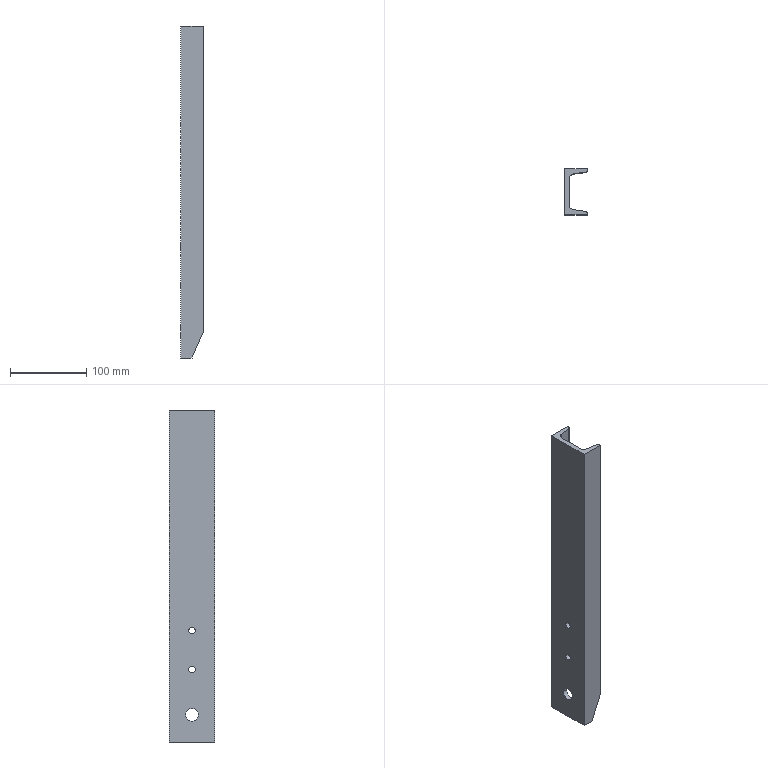Part | SolidWorks | features ICE 3, Extrusion 1 | 1 solid | 22 faces | box 30 x 60 x 435 mm | volume 272325 mm3 | plane 12 | cylinder 10 | commonest cylinder face diameters 8.5 x4 6 x2 12 x2 17 x2
STEP:
#1=CARTESIAN_POINT('',(-24.,-25.75,95.));
#2=VERTEX_POINT('',#1);
#3=CARTESIAN_POINT('',(-24.,-34.25,95.));
#4=VERTEX_POINT('',#3);
#5=CARTESIAN_POINT('',(-24.,-30.,95.));
#6=DIRECTION('',(-1.,0.,0.));
#7=DIRECTION('',(0.,0.,1.));
#8=AXIS2_PLACEMENT_3D('',#5,#6,#7);
#9=CIRCLE('',#8,4.25);
#10=EDGE_CURVE('',#2,#4,#9,.T.);
#11=ORIENTED_EDGE('',*,*,#10,.F.);
#12=CARTESIAN_POINT('',(-30.,-25.75,95.));
#13=VERTEX_POINT('',#12);
#14=CARTESIAN_POINT('',(405.,-25.75,95.));
#15=DIRECTION('',(-1.,0.,0.));
#16=VECTOR('',#15,1000.);
#17=LINE('',#14,#16);
#18=EDGE_CURVE('',#2,#13,#17,.T.);
#19=ORIENTED_EDGE('',*,*,#18,.T.);
#20=CARTESIAN_POINT('',(-30.,-34.25,95.));
#21=VERTEX_POINT('',#20);
#22=CARTESIAN_POINT('',(-30.,-30.,95.));
#23=DIRECTION('',(-1.,0.,0.));
#24=DIRECTION('',(0.,-1.,0.));
#25=AXIS2_PLACEMENT_3D('',#22,#23,#24);
#26=CIRCLE('',#25,4.25);
#27=EDGE_CURVE('',#13,#21,#26,.T.);
#28=ORIENTED_EDGE('',*,*,#27,.T.);
#29=CARTESIAN_POINT('',(405.,-34.25,95.));
#30=DIRECTION('',(-1.,0.,0.));
#31=VECTOR('',#30,1000.);
#32=LINE('',#29,#31);
#33=EDGE_CURVE('',#4,#21,#32,.T.);
#34=ORIENTED_EDGE('',*,*,#33,.F.);
#35=EDGE_LOOP('',(#11,#19,#28,#34));
#36=FACE_OUTER_BOUND('',#35,.T.);
#37=CARTESIAN_POINT('',(405.,-30.,95.));
#38=DIRECTION('',(-1.,0.,0.));
#39=DIRECTION('',(0.,-1.,0.));
#40=AXIS2_PLACEMENT_3D('',#37,#38,#39);
#41=CYLINDRICAL_SURFACE('',#40,4.25);
#42=ADVANCED_FACE('',(#36),#41,.F.);
#43=CARTESIAN_POINT('',(-24.,-25.75,146.));
#44=VERTEX_POINT('',#43);
#45=CARTESIAN_POINT('',(-24.,-34.25,146.));
#46=VERTEX_POINT('',#45);
#47=CARTESIAN_POINT('',(-24.,-30.,146.));
#48=DIRECTION('',(-1.,0.,0.));
#49=DIRECTION('',(0.,0.,1.));
#50=AXIS2_PLACEMENT_3D('',#47,#48,#49);
#51=CIRCLE('',#50,4.25);
#52=EDGE_CURVE('',#44,#46,#51,.T.);
#53=ORIENTED_EDGE('',*,*,#52,.F.);
#54=CARTESIAN_POINT('',(-30.,-25.75,146.));
#55=VERTEX_POINT('',#54);
#56=CARTESIAN_POINT('',(405.,-25.75,146.));
#57=DIRECTION('',(-1.,0.,0.));
#58=VECTOR('',#57,1000.);
#59=LINE('',#56,#58);
#60=EDGE_CURVE('',#44,#55,#59,.T.);
#61=ORIENTED_EDGE('',*,*,#60,.T.);
#62=CARTESIAN_POINT('',(-30.,-34.25,146.));
#63=VERTEX_POINT('',#62);
#64=CARTESIAN_POINT('',(-30.,-30.,146.));
#65=DIRECTION('',(-1.,0.,0.));
#66=DIRECTION('',(0.,-1.,0.));
#67=AXIS2_PLACEMENT_3D('',#64,#65,#66);
#68=CIRCLE('',#67,4.25);
#69=EDGE_CURVE('',#55,#63,#68,.T.);
#70=ORIENTED_EDGE('',*,*,#69,.T.);
#71=CARTESIAN_POINT('',(405.,-34.25,146.));
#72=DIRECTION('',(-1.,0.,0.));
#73=VECTOR('',#72,1000.);
#74=LINE('',#71,#73);
#75=EDGE_CURVE('',#46,#63,#74,.T.);
#76=ORIENTED_EDGE('',*,*,#75,.F.);
#77=EDGE_LOOP('',(#53,#61,#70,#76));
#78=FACE_OUTER_BOUND('',#77,.T.);
#79=CARTESIAN_POINT('',(405.,-30.,146.));
#80=DIRECTION('',(-1.,0.,0.));
#81=DIRECTION('',(0.,-1.,0.));
#82=AXIS2_PLACEMENT_3D('',#79,#80,#81);
#83=CYLINDRICAL_SURFACE('',#82,4.25);
#84=ADVANCED_FACE('',(#78),#83,.F.);
#85=CARTESIAN_POINT('',(-24.,-21.5,35.5));
#86=VERTEX_POINT('',#85);
#87=CARTESIAN_POINT('',(-24.,-38.5,35.5));
#88=VERTEX_POINT('',#87);
#89=CARTESIAN_POINT('',(-24.,-30.,35.5));
#90=DIRECTION('',(-1.,0.,0.));
#91=DIRECTION('',(0.,0.,1.));
#92=AXIS2_PLACEMENT_3D('',#89,#90,#91);
#93=CIRCLE('',#92,8.5);
#94=EDGE_CURVE('',#86,#88,#93,.T.);
#95=ORIENTED_EDGE('',*,*,#94,.F.);
#96=CARTESIAN_POINT('',(-30.,-21.5,35.5));
#97=VERTEX_POINT('',#96);
#98=CARTESIAN_POINT('',(405.,-21.5,35.5));
#99=DIRECTION('',(-1.,0.,0.));
#100=VECTOR('',#99,1000.);
#101=LINE('',#98,#100);
#102=EDGE_CURVE('',#86,#97,#101,.T.);
#103=ORIENTED_EDGE('',*,*,#102,.T.);
#104=CARTESIAN_POINT('',(-30.,-38.5,35.5));
#105=VERTEX_POINT('',#104);
#106=CARTESIAN_POINT('',(-30.,-30.,35.5));
#107=DIRECTION('',(-1.,0.,0.));
#108=DIRECTION('',(0.,-1.,0.));
#109=AXIS2_PLACEMENT_3D('',#106,#107,#108);
#110=CIRCLE('',#109,8.5);
#111=EDGE_CURVE('',#97,#105,#110,.T.);
#112=ORIENTED_EDGE('',*,*,#111,.T.);
#113=CARTESIAN_POINT('',(405.,-38.5,35.5));
#114=DIRECTION('',(-1.,0.,0.));
#115=VECTOR('',#114,1000.);
#116=LINE('',#113,#115);
#117=EDGE_CURVE('',#88,#105,#116,.T.);
#118=ORIENTED_EDGE('',*,*,#117,.F.);
#119=EDGE_LOOP('',(#95,#103,#112,#118));
#120=FACE_OUTER_BOUND('',#119,.T.);
#121=CARTESIAN_POINT('',(405.,-30.,35.5));
#122=DIRECTION('',(-1.,0.,0.));
#123=DIRECTION('',(0.,-1.,0.));
#124=AXIS2_PLACEMENT_3D('',#121,#122,#123);
#125=CYLINDRICAL_SURFACE('',#124,8.5);
#126=ADVANCED_FACE('',(#120),#125,.F.);
#127=CARTESIAN_POINT('',(0.,-1.284,435.));
#128=VERTEX_POINT('',#127);
#129=CARTESIAN_POINT('',(0.,-1.284,35.));
#130=VERTEX_POINT('',#129);
#131=CARTESIAN_POINT('',(0.,-1.284,435.));
#132=DIRECTION('',(0.,0.,-1.));
#133=VECTOR('',#132,1000.);
#134=LINE('',#131,#133);
#135=EDGE_CURVE('',#128,#130,#134,.T.);
#136=ORIENTED_EDGE('',*,*,#135,.T.);
#137=CARTESIAN_POINT('',(0.,0.,35.));
#138=VERTEX_POINT('',#137);
#139=CARTESIAN_POINT('',(0.,-435.,35.));
#140=DIRECTION('',(0.,1.,0.));
#141=VECTOR('',#140,1000.);
#142=LINE('',#139,#141);
#143=EDGE_CURVE('',#130,#138,#142,.T.);
#144=ORIENTED_EDGE('',*,*,#143,.T.);
#145=CARTESIAN_POINT('',(0.,0.,435.));
#146=VERTEX_POINT('',#145);
#147=CARTESIAN_POINT('',(0.,0.,435.));
#148=DIRECTION('',(0.,0.,-1.));
#149=VECTOR('',#148,1000.);
#150=LINE('',#147,#149);
#151=EDGE_CURVE('',#146,#138,#150,.T.);
#152=ORIENTED_EDGE('',*,*,#151,.F.);
#153=CARTESIAN_POINT('',(0.,-1.284,435.));
#154=DIRECTION('',(0.,1.,0.));
#155=VECTOR('',#154,1000.);
#156=LINE('',#153,#155);
#157=EDGE_CURVE('',#128,#146,#156,.T.);
#158=ORIENTED_EDGE('',*,*,#157,.F.);
#159=EDGE_LOOP('',(#136,#144,#152,#158));
#160=FACE_OUTER_BOUND('',#159,.T.);
#161=CARTESIAN_POINT('',(0.,-1.284,435.));
#162=DIRECTION('',(-1.,0.,0.));
#163=DIRECTION('',(0.,0.,1.));
#164=AXIS2_PLACEMENT_3D('',#161,#162,#163);
#165=PLANE('',#164);
#166=ADVANCED_FACE('',(#160),#165,.F.);
#167=ORIENTED_EDGE('',*,*,#151,.T.);
#168=CARTESIAN_POINT('',(-15.,0.,0.));
#169=VERTEX_POINT('',#168);
#170=CARTESIAN_POINT('',(0.,0.,35.));
#171=DIRECTION('',(0.3939,0.,0.9191));
#172=VECTOR('',#171,1000.);
#173=LINE('',#170,#172);
#174=EDGE_CURVE('',#169,#138,#173,.T.);
#175=ORIENTED_EDGE('',*,*,#174,.F.);
#176=CARTESIAN_POINT('',(-30.,0.,0.));
#177=VERTEX_POINT('',#176);
#178=CARTESIAN_POINT('',(0.,0.,0.));
#179=DIRECTION('',(-1.,0.,0.));
#180=VECTOR('',#179,1000.);
#181=LINE('',#178,#180);
#182=EDGE_CURVE('',#169,#177,#181,.T.);
#183=ORIENTED_EDGE('',*,*,#182,.T.);
#184=CARTESIAN_POINT('',(-30.,0.,435.));
#185=VERTEX_POINT('',#184);
#186=CARTESIAN_POINT('',(-30.,0.,435.));
#187=DIRECTION('',(0.,0.,-1.));
#188=VECTOR('',#187,1000.);
#189=LINE('',#186,#188);
#190=EDGE_CURVE('',#185,#177,#189,.T.);
#191=ORIENTED_EDGE('',*,*,#190,.F.);
#192=CARTESIAN_POINT('',(0.,0.,435.));
#193=DIRECTION('',(-1.,0.,0.));
#194=VECTOR('',#193,1000.);
#195=LINE('',#192,#194);
#196=EDGE_CURVE('',#146,#185,#195,.T.);
#197=ORIENTED_EDGE('',*,*,#196,.F.);
#198=EDGE_LOOP('',(#167,#175,#183,#191,#197));
#199=FACE_OUTER_BOUND('',#198,.T.);
#200=CARTESIAN_POINT('',(0.,0.,435.));
#201=DIRECTION('',(0.,-1.,0.));
#202=DIRECTION('',(1.,0.,0.));
#203=AXIS2_PLACEMENT_3D('',#200,#201,#202);
#204=PLANE('',#203);
#205=ADVANCED_FACE('',(#199),#204,.F.);
#206=CARTESIAN_POINT('',(-30.,-30.,95.));
#207=DIRECTION('',(-1.,0.,0.));
#208=DIRECTION('',(0.,-1.,0.));
#209=AXIS2_PLACEMENT_3D('',#206,#207,#208);
#210=CIRCLE('',#209,4.25);
#211=EDGE_CURVE('',#21,#13,#210,.T.);
#212=ORIENTED_EDGE('',*,*,#211,.F.);
#213=ORIENTED_EDGE('',*,*,#27,.F.);
#214=EDGE_LOOP('',(#212,#213));
#215=FACE_BOUND('',#214,.T.);
#216=CARTESIAN_POINT('',(-30.,-30.,146.));
#217=DIRECTION('',(-1.,0.,0.));
#218=DIRECTION('',(0.,-1.,0.));
#219=AXIS2_PLACEMENT_3D('',#216,#217,#218);
#220=CIRCLE('',#219,4.25);
#221=EDGE_CURVE('',#63,#55,#220,.T.);
#222=ORIENTED_EDGE('',*,*,#221,.F.);
#223=ORIENTED_EDGE('',*,*,#69,.F.);
#224=EDGE_LOOP('',(#222,#223));
#225=FACE_BOUND('',#224,.T.);
#226=CARTESIAN_POINT('',(-30.,-30.,35.5));
#227=DIRECTION('',(-1.,0.,0.));
#228=DIRECTION('',(0.,-1.,0.));
#229=AXIS2_PLACEMENT_3D('',#226,#227,#228);
#230=CIRCLE('',#229,8.5);
#231=EDGE_CURVE('',#105,#97,#230,.T.);
#232=ORIENTED_EDGE('',*,*,#231,.F.);
#233=ORIENTED_EDGE('',*,*,#111,.F.);
#234=EDGE_LOOP('',(#232,#233));
#235=FACE_BOUND('',#234,.T.);
#236=CARTESIAN_POINT('',(-30.,-60.,0.));
#237=VERTEX_POINT('',#236);
#238=CARTESIAN_POINT('',(-30.,0.,0.));
#239=DIRECTION('',(0.,-1.,0.));
#240=VECTOR('',#239,1000.);
#241=LINE('',#238,#240);
#242=EDGE_CURVE('',#177,#237,#241,.T.);
#243=ORIENTED_EDGE('',*,*,#242,.T.);
#244=CARTESIAN_POINT('',(-30.,-60.,435.));
#245=VERTEX_POINT('',#244);
#246=CARTESIAN_POINT('',(-30.,-60.,435.));
#247=DIRECTION('',(0.,0.,-1.));
#248=VECTOR('',#247,1000.);
#249=LINE('',#246,#248);
#250=EDGE_CURVE('',#245,#237,#249,.T.);
#251=ORIENTED_EDGE('',*,*,#250,.F.);
#252=CARTESIAN_POINT('',(-30.,0.,435.));
#253=DIRECTION('',(0.,-1.,0.));
#254=VECTOR('',#253,1000.);
#255=LINE('',#252,#254);
#256=EDGE_CURVE('',#185,#245,#255,.T.);
#257=ORIENTED_EDGE('',*,*,#256,.F.);
#258=ORIENTED_EDGE('',*,*,#190,.T.);
#259=EDGE_LOOP('',(#243,#251,#257,#258));
#260=FACE_OUTER_BOUND('',#259,.T.);
#261=CARTESIAN_POINT('',(-30.,0.,435.));
#262=DIRECTION('',(1.,0.,0.));
#263=DIRECTION('',(0.,1.,0.));
#264=AXIS2_PLACEMENT_3D('',#261,#262,#263);
#265=PLANE('',#264);
#266=ADVANCED_FACE('',(#215,#225,#235,#260),#265,.F.);
#267=CARTESIAN_POINT('',(-15.,-60.,0.));
#268=VERTEX_POINT('',#267);
#269=CARTESIAN_POINT('',(-30.,-60.,0.));
#270=DIRECTION('',(1.,0.,0.));
#271=VECTOR('',#270,1000.);
#272=LINE('',#269,#271);
#273=EDGE_CURVE('',#237,#268,#272,.T.);
#274=ORIENTED_EDGE('',*,*,#273,.T.);
#275=CARTESIAN_POINT('',(0.,-60.,35.));
#276=VERTEX_POINT('',#275);
#277=CARTESIAN_POINT('',(140.172,-60.,362.069));
#278=DIRECTION('',(0.3939,0.,0.9191));
#279=VECTOR('',#278,1000.);
#280=LINE('',#277,#279);
#281=EDGE_CURVE('',#268,#276,#280,.T.);
#282=ORIENTED_EDGE('',*,*,#281,.T.);
#283=CARTESIAN_POINT('',(0.,-60.,435.));
#284=VERTEX_POINT('',#283);
#285=CARTESIAN_POINT('',(0.,-60.,435.));
#286=DIRECTION('',(0.,0.,-1.));
#287=VECTOR('',#286,1000.);
#288=LINE('',#285,#287);
#289=EDGE_CURVE('',#284,#276,#288,.T.);
#290=ORIENTED_EDGE('',*,*,#289,.F.);
#291=CARTESIAN_POINT('',(-30.,-60.,435.));
#292=DIRECTION('',(1.,0.,0.));
#293=VECTOR('',#292,1000.);
#294=LINE('',#291,#293);
#295=EDGE_CURVE('',#245,#284,#294,.T.);
#296=ORIENTED_EDGE('',*,*,#295,.F.);
#297=ORIENTED_EDGE('',*,*,#250,.T.);
#298=EDGE_LOOP('',(#274,#282,#290,#296,#297));
#299=FACE_OUTER_BOUND('',#298,.T.);
#300=CARTESIAN_POINT('',(-30.,-60.,435.));
#301=DIRECTION('',(0.,1.,0.));
#302=DIRECTION('',(-1.,0.,0.));
#303=AXIS2_PLACEMENT_3D('',#300,#301,#302);
#304=PLANE('',#303);
#305=ADVANCED_FACE('',(#299),#304,.F.);
#306=ORIENTED_EDGE('',*,*,#289,.T.);
#307=CARTESIAN_POINT('',(0.,-58.716,35.));
#308=VERTEX_POINT('',#307);
#309=CARTESIAN_POINT('',(0.,-435.,35.));
#310=DIRECTION('',(0.,1.,0.));
#311=VECTOR('',#310,1000.);
#312=LINE('',#309,#311);
#313=EDGE_CURVE('',#276,#308,#312,.T.);
#314=ORIENTED_EDGE('',*,*,#313,.T.);
#315=CARTESIAN_POINT('',(0.,-58.716,435.));
#316=VERTEX_POINT('',#315);
#317=CARTESIAN_POINT('',(0.,-58.716,435.));
#318=DIRECTION('',(0.,0.,-1.));
#319=VECTOR('',#318,1000.);
#320=LINE('',#317,#319);
#321=EDGE_CURVE('',#316,#308,#320,.T.);
#322=ORIENTED_EDGE('',*,*,#321,.F.);
#323=CARTESIAN_POINT('',(0.,-60.,435.));
#324=DIRECTION('',(0.,1.,0.));
#325=VECTOR('',#324,1000.);
#326=LINE('',#323,#325);
#327=EDGE_CURVE('',#284,#316,#326,.T.);
#328=ORIENTED_EDGE('',*,*,#327,.F.);
#329=EDGE_LOOP('',(#306,#314,#322,#328));
#330=FACE_OUTER_BOUND('',#329,.T.);
#331=CARTESIAN_POINT('',(0.,-60.,435.));
#332=DIRECTION('',(-1.,0.,0.));
#333=DIRECTION('',(0.,0.,1.));
#334=AXIS2_PLACEMENT_3D('',#331,#332,#333);
#335=PLANE('',#334);
#336=ADVANCED_FACE('',(#330),#335,.F.);
#337=ORIENTED_EDGE('',*,*,#321,.T.);
#338=CARTESIAN_POINT('',(-2.582,-55.745,28.974));
#339=VERTEX_POINT('',#338);
#340=CARTESIAN_POINT('',(0.,-58.716,35.));
#341=CARTESIAN_POINT('',(0.,-57.147,35.));
#342=CARTESIAN_POINT('',(-1.029,-55.963,32.599));
#343=CARTESIAN_POINT('',(-2.582,-55.745,28.974));
#344=(BOUNDED_CURVE()B_SPLINE_CURVE(3,(#340,#341,#342,#343),.UNSPECIFIED.,.F.,.T.)B_SPLINE_CURVE_WITH_KNOTS((4,4),(3.142,4.573),.UNSPECIFIED.)CURVE()GEOMETRIC_REPRESENTATION_ITEM()RATIONAL_B_SPLINE_CURVE((1.,0.8365,0.8365,1.))REPRESENTATION_ITEM(''));
#345=EDGE_CURVE('',#308,#339,#344,.T.);
#346=ORIENTED_EDGE('',*,*,#345,.T.);
#347=CARTESIAN_POINT('',(-2.582,-55.745,435.));
#348=VERTEX_POINT('',#347);
#349=CARTESIAN_POINT('',(-2.582,-55.745,435.));
#350=DIRECTION('',(0.,0.,-1.));
#351=VECTOR('',#350,1000.);
#352=LINE('',#349,#351);
#353=EDGE_CURVE('',#348,#339,#352,.T.);
#354=ORIENTED_EDGE('',*,*,#353,.F.);
#355=CARTESIAN_POINT('',(-3.,-58.716,435.));
#356=DIRECTION('',(0.,0.,1.));
#357=DIRECTION('',(1.,0.,0.));
#358=AXIS2_PLACEMENT_3D('',#355,#356,#357);
#359=CIRCLE('',#358,3.);
#360=EDGE_CURVE('',#316,#348,#359,.T.);
#361=ORIENTED_EDGE('',*,*,#360,.F.);
#362=EDGE_LOOP('',(#337,#346,#354,#361));
#363=FACE_OUTER_BOUND('',#362,.T.);
#364=CARTESIAN_POINT('',(-3.,-58.716,435.));
#365=DIRECTION('',(0.,0.,-1.));
#366=DIRECTION('',(-1.,0.,0.));
#367=AXIS2_PLACEMENT_3D('',#364,#365,#366);
#368=CYLINDRICAL_SURFACE('',#367,3.);
#369=ADVANCED_FACE('',(#363),#368,.T.);
#370=ORIENTED_EDGE('',*,*,#353,.T.);
#371=CARTESIAN_POINT('',(-15.,-54.,0.));
#372=VERTEX_POINT('',#371);
#373=CARTESIAN_POINT('',(143.978,-76.343,370.948));
#374=DIRECTION('',(-0.3933,0.05528,-0.9177));
#375=VECTOR('',#374,1000.);
#376=LINE('',#373,#375);
#377=EDGE_CURVE('',#339,#372,#376,.T.);
#378=ORIENTED_EDGE('',*,*,#377,.T.);
#379=CARTESIAN_POINT('',(-18.835,-53.461,0.));
#380=VERTEX_POINT('',#379);
#381=CARTESIAN_POINT('',(-2.582,-55.745,0.));
#382=DIRECTION('',(-0.9903,0.1392,0.));
#383=VECTOR('',#382,1000.);
#384=LINE('',#381,#383);
#385=EDGE_CURVE('',#372,#380,#384,.T.);
#386=ORIENTED_EDGE('',*,*,#385,.T.);
#387=CARTESIAN_POINT('',(-18.835,-53.461,435.));
#388=VERTEX_POINT('',#387);
#389=CARTESIAN_POINT('',(-18.835,-53.461,435.));
#390=DIRECTION('',(0.,0.,-1.));
#391=VECTOR('',#390,1000.);
#392=LINE('',#389,#391);
#393=EDGE_CURVE('',#388,#380,#392,.T.);
#394=ORIENTED_EDGE('',*,*,#393,.F.);
#395=CARTESIAN_POINT('',(-2.582,-55.745,435.));
#396=DIRECTION('',(-0.9903,0.1392,0.));
#397=VECTOR('',#396,1000.);
#398=LINE('',#395,#397);
#399=EDGE_CURVE('',#348,#388,#398,.T.);
#400=ORIENTED_EDGE('',*,*,#399,.F.);
#401=EDGE_LOOP('',(#370,#378,#386,#394,#400));
#402=FACE_OUTER_BOUND('',#401,.T.);
#403=CARTESIAN_POINT('',(-2.582,-55.745,435.));
#404=DIRECTION('',(-0.1392,-0.9903,0.));
#405=DIRECTION('',(0.9903,-0.1392,0.));
#406=AXIS2_PLACEMENT_3D('',#403,#404,#405);
#407=PLANE('',#406);
#408=ADVANCED_FACE('',(#402),#407,.F.);
#409=CARTESIAN_POINT('',(-24.,-47.519,0.));
#410=VERTEX_POINT('',#409);
#411=CARTESIAN_POINT('',(-18.,-47.519,0.));
#412=DIRECTION('',(0.,0.,-1.));
#413=DIRECTION('',(-1.,0.,0.));
#414=AXIS2_PLACEMENT_3D('',#411,#412,#413);
#415=CIRCLE('',#414,6.);
#416=EDGE_CURVE('',#380,#410,#415,.T.);
#417=ORIENTED_EDGE('',*,*,#416,.T.);
#418=CARTESIAN_POINT('',(-24.,-47.519,435.));
#419=VERTEX_POINT('',#418);
#420=CARTESIAN_POINT('',(-24.,-47.519,435.));
#421=DIRECTION('',(0.,0.,-1.));
#422=VECTOR('',#421,1000.);
#423=LINE('',#420,#422);
#424=EDGE_CURVE('',#419,#410,#423,.T.);
#425=ORIENTED_EDGE('',*,*,#424,.F.);
#426=CARTESIAN_POINT('',(-18.,-47.519,435.));
#427=DIRECTION('',(0.,0.,-1.));
#428=DIRECTION('',(-1.,0.,0.));
#429=AXIS2_PLACEMENT_3D('',#426,#427,#428);
#430=CIRCLE('',#429,6.);
#431=EDGE_CURVE('',#388,#419,#430,.T.);
#432=ORIENTED_EDGE('',*,*,#431,.F.);
#433=ORIENTED_EDGE('',*,*,#393,.T.);
#434=EDGE_LOOP('',(#417,#425,#432,#433));
#435=FACE_OUTER_BOUND('',#434,.T.);
#436=CARTESIAN_POINT('',(-18.,-47.519,435.));
#437=DIRECTION('',(0.,0.,-1.));
#438=DIRECTION('',(-1.,0.,0.));
#439=AXIS2_PLACEMENT_3D('',#436,#437,#438);
#440=CYLINDRICAL_SURFACE('',#439,6.);
#441=ADVANCED_FACE('',(#435),#440,.F.);
#442=CARTESIAN_POINT('',(-24.,-30.,95.));
#443=DIRECTION('',(-1.,0.,0.));
#444=DIRECTION('',(0.,0.,1.));
#445=AXIS2_PLACEMENT_3D('',#442,#443,#444);
#446=CIRCLE('',#445,4.25);
#447=EDGE_CURVE('',#4,#2,#446,.T.);
#448=ORIENTED_EDGE('',*,*,#447,.T.);
#449=ORIENTED_EDGE('',*,*,#10,.T.);
#450=EDGE_LOOP('',(#448,#449));
#451=FACE_BOUND('',#450,.T.);
#452=CARTESIAN_POINT('',(-24.,-30.,146.));
#453=DIRECTION('',(-1.,0.,0.));
#454=DIRECTION('',(0.,0.,1.));
#455=AXIS2_PLACEMENT_3D('',#452,#453,#454);
#456=CIRCLE('',#455,4.25);
#457=EDGE_CURVE('',#46,#44,#456,.T.);
#458=ORIENTED_EDGE('',*,*,#457,.T.);
#459=ORIENTED_EDGE('',*,*,#52,.T.);
#460=EDGE_LOOP('',(#458,#459));
#461=FACE_BOUND('',#460,.T.);
#462=CARTESIAN_POINT('',(-24.,-30.,35.5));
#463=DIRECTION('',(-1.,0.,0.));
#464=DIRECTION('',(0.,0.,1.));
#465=AXIS2_PLACEMENT_3D('',#462,#463,#464);
#466=CIRCLE('',#465,8.5);
#467=EDGE_CURVE('',#88,#86,#466,.T.);
#468=ORIENTED_EDGE('',*,*,#467,.T.);
#469=ORIENTED_EDGE('',*,*,#94,.T.);
#470=EDGE_LOOP('',(#468,#469));
#471=FACE_BOUND('',#470,.T.);
#472=CARTESIAN_POINT('',(-24.,-12.481,0.));
#473=VERTEX_POINT('',#472);
#474=CARTESIAN_POINT('',(-24.,-47.519,0.));
#475=DIRECTION('',(0.,1.,0.));
#476=VECTOR('',#475,1000.);
#477=LINE('',#474,#476);
#478=EDGE_CURVE('',#410,#473,#477,.T.);
#479=ORIENTED_EDGE('',*,*,#478,.T.);
#480=CARTESIAN_POINT('',(-24.,-12.481,435.));
#481=VERTEX_POINT('',#480);
#482=CARTESIAN_POINT('',(-24.,-12.481,435.));
#483=DIRECTION('',(0.,0.,-1.));
#484=VECTOR('',#483,1000.);
#485=LINE('',#482,#484);
#486=EDGE_CURVE('',#481,#473,#485,.T.);
#487=ORIENTED_EDGE('',*,*,#486,.F.);
#488=CARTESIAN_POINT('',(-24.,-47.519,435.));
#489=DIRECTION('',(0.,1.,0.));
#490=VECTOR('',#489,1000.);
#491=LINE('',#488,#490);
#492=EDGE_CURVE('',#419,#481,#491,.T.);
#493=ORIENTED_EDGE('',*,*,#492,.F.);
#494=ORIENTED_EDGE('',*,*,#424,.T.);
#495=EDGE_LOOP('',(#479,#487,#493,#494));
#496=FACE_OUTER_BOUND('',#495,.T.);
#497=CARTESIAN_POINT('',(-24.,-47.519,435.));
#498=DIRECTION('',(-1.,0.,0.));
#499=DIRECTION('',(0.,0.,1.));
#500=AXIS2_PLACEMENT_3D('',#497,#498,#499);
#501=PLANE('',#500);
#502=ADVANCED_FACE('',(#451,#461,#471,#496),#501,.F.);
#503=CARTESIAN_POINT('',(-18.835,-6.539,0.));
#504=VERTEX_POINT('',#503);
#505=CARTESIAN_POINT('',(-18.,-12.481,0.));
#506=DIRECTION('',(0.,0.,-1.));
#507=DIRECTION('',(-1.,0.,0.));
#508=AXIS2_PLACEMENT_3D('',#505,#506,#507);
#509=CIRCLE('',#508,6.);
#510=EDGE_CURVE('',#473,#504,#509,.T.);
#511=ORIENTED_EDGE('',*,*,#510,.T.);
#512=CARTESIAN_POINT('',(-18.835,-6.539,435.));
#513=VERTEX_POINT('',#512);
#514=CARTESIAN_POINT('',(-18.835,-6.539,435.));
#515=DIRECTION('',(0.,0.,-1.));
#516=VECTOR('',#515,1000.);
#517=LINE('',#514,#516);
#518=EDGE_CURVE('',#513,#504,#517,.T.);
#519=ORIENTED_EDGE('',*,*,#518,.F.);
#520=CARTESIAN_POINT('',(-18.,-12.481,435.));
#521=DIRECTION('',(0.,0.,-1.));
#522=DIRECTION('',(-1.,0.,0.));
#523=AXIS2_PLACEMENT_3D('',#520,#521,#522);
#524=CIRCLE('',#523,6.);
#525=EDGE_CURVE('',#481,#513,#524,.T.);
#526=ORIENTED_EDGE('',*,*,#525,.F.);
#527=ORIENTED_EDGE('',*,*,#486,.T.);
#528=EDGE_LOOP('',(#511,#519,#526,#527));
#529=FACE_OUTER_BOUND('',#528,.T.);
#530=CARTESIAN_POINT('',(-18.,-12.481,435.));
#531=DIRECTION('',(0.,0.,-1.));
#532=DIRECTION('',(-1.,0.,0.));
#533=AXIS2_PLACEMENT_3D('',#530,#531,#532);
#534=CYLINDRICAL_SURFACE('',#533,6.);
#535=ADVANCED_FACE('',(#529),#534,.F.);
#536=CARTESIAN_POINT('',(-15.,-6.,0.));
#537=VERTEX_POINT('',#536);
#538=CARTESIAN_POINT('',(-18.835,-6.539,0.));
#539=DIRECTION('',(0.9903,0.1392,0.));
#540=VECTOR('',#539,1000.);
#541=LINE('',#538,#540);
#542=EDGE_CURVE('',#504,#537,#541,.T.);
#543=ORIENTED_EDGE('',*,*,#542,.T.);
#544=CARTESIAN_POINT('',(-2.582,-4.255,28.974));
#545=VERTEX_POINT('',#544);
#546=CARTESIAN_POINT('',(141.414,15.983,364.965));
#547=DIRECTION('',(0.3933,0.05528,0.9177));
#548=VECTOR('',#547,1000.);
#549=LINE('',#546,#548);
#550=EDGE_CURVE('',#537,#545,#549,.T.);
#551=ORIENTED_EDGE('',*,*,#550,.T.);
#552=CARTESIAN_POINT('',(-2.582,-4.255,435.));
#553=VERTEX_POINT('',#552);
#554=CARTESIAN_POINT('',(-2.582,-4.255,435.));
#555=DIRECTION('',(0.,0.,-1.));
#556=VECTOR('',#555,1000.);
#557=LINE('',#554,#556);
#558=EDGE_CURVE('',#553,#545,#557,.T.);
#559=ORIENTED_EDGE('',*,*,#558,.F.);
#560=CARTESIAN_POINT('',(-18.835,-6.539,435.));
#561=DIRECTION('',(0.9903,0.1392,0.));
#562=VECTOR('',#561,1000.);
#563=LINE('',#560,#562);
#564=EDGE_CURVE('',#513,#553,#563,.T.);
#565=ORIENTED_EDGE('',*,*,#564,.F.);
#566=ORIENTED_EDGE('',*,*,#518,.T.);
#567=EDGE_LOOP('',(#543,#551,#559,#565,#566));
#568=FACE_OUTER_BOUND('',#567,.T.);
#569=CARTESIAN_POINT('',(-18.835,-6.539,435.));
#570=DIRECTION('',(-0.1392,0.9903,0.));
#571=DIRECTION('',(-0.9903,-0.1392,0.));
#572=AXIS2_PLACEMENT_3D('',#569,#570,#571);
#573=PLANE('',#572);
#574=ADVANCED_FACE('',(#568),#573,.F.);
#575=CARTESIAN_POINT('',(0.,-1.284,35.));
#576=CARTESIAN_POINT('',(0.,-2.853,35.));
#577=CARTESIAN_POINT('',(-1.029,-4.037,32.599));
#578=CARTESIAN_POINT('',(-2.582,-4.255,28.974));
#579=(BOUNDED_CURVE()B_SPLINE_CURVE(3,(#575,#576,#577,#578),.UNSPECIFIED.,.F.,.T.)B_SPLINE_CURVE_WITH_KNOTS((4,4),(3.142,4.573),.UNSPECIFIED.)CURVE()GEOMETRIC_REPRESENTATION_ITEM()RATIONAL_B_SPLINE_CURVE((1.,0.8365,0.8365,1.))REPRESENTATION_ITEM(''));
#580=EDGE_CURVE('',#130,#545,#579,.T.);
#581=ORIENTED_EDGE('',*,*,#580,.F.);
#582=ORIENTED_EDGE('',*,*,#135,.F.);
#583=CARTESIAN_POINT('',(-3.,-1.284,435.));
#584=DIRECTION('',(0.,0.,-1.));
#585=DIRECTION('',(-1.,0.,0.));
#586=AXIS2_PLACEMENT_3D('',#583,#584,#585);
#587=CIRCLE('',#586,3.);
#588=EDGE_CURVE('',#128,#553,#587,.T.);
#589=ORIENTED_EDGE('',*,*,#588,.T.);
#590=ORIENTED_EDGE('',*,*,#558,.T.);
#591=EDGE_LOOP('',(#581,#582,#589,#590));
#592=FACE_OUTER_BOUND('',#591,.T.);
#593=CARTESIAN_POINT('',(-3.,-1.284,435.));
#594=DIRECTION('',(0.,0.,-1.));
#595=DIRECTION('',(-1.,0.,0.));
#596=AXIS2_PLACEMENT_3D('',#593,#594,#595);
#597=CYLINDRICAL_SURFACE('',#596,3.);
#598=ADVANCED_FACE('',(#592),#597,.T.);
#599=ORIENTED_EDGE('',*,*,#157,.T.);
#600=ORIENTED_EDGE('',*,*,#196,.T.);
#601=ORIENTED_EDGE('',*,*,#256,.T.);
#602=ORIENTED_EDGE('',*,*,#295,.T.);
#603=ORIENTED_EDGE('',*,*,#327,.T.);
#604=ORIENTED_EDGE('',*,*,#360,.T.);
#605=ORIENTED_EDGE('',*,*,#399,.T.);
#606=ORIENTED_EDGE('',*,*,#431,.T.);
#607=ORIENTED_EDGE('',*,*,#492,.T.);
#608=ORIENTED_EDGE('',*,*,#525,.T.);
#609=ORIENTED_EDGE('',*,*,#564,.T.);
#610=ORIENTED_EDGE('',*,*,#588,.F.);
#611=EDGE_LOOP('',(#599,#600,#601,#602,#603,#604,#605,#606,#607,#608,#609,#610));
#612=FACE_OUTER_BOUND('',#611,.T.);
#613=CARTESIAN_POINT('',(-3.,-58.716,435.));
#614=DIRECTION('',(0.,0.,1.));
#615=DIRECTION('',(1.,0.,0.));
#616=AXIS2_PLACEMENT_3D('',#613,#614,#615);
#617=PLANE('',#616);
#618=ADVANCED_FACE('',(#612),#617,.T.);
#619=ORIENTED_EDGE('',*,*,#182,.F.);
#620=CARTESIAN_POINT('',(-15.,-58.716,0.));
#621=DIRECTION('',(0.,-1.,0.));
#622=VECTOR('',#621,1000.);
#623=LINE('',#620,#622);
#624=EDGE_CURVE('',#169,#537,#623,.T.);
#625=ORIENTED_EDGE('',*,*,#624,.T.);
#626=ORIENTED_EDGE('',*,*,#542,.F.);
#627=ORIENTED_EDGE('',*,*,#510,.F.);
#628=ORIENTED_EDGE('',*,*,#478,.F.);
#629=ORIENTED_EDGE('',*,*,#416,.F.);
#630=ORIENTED_EDGE('',*,*,#385,.F.);
#631=CARTESIAN_POINT('',(-15.,-58.716,0.));
#632=DIRECTION('',(0.,-1.,0.));
#633=VECTOR('',#632,1000.);
#634=LINE('',#631,#633);
#635=EDGE_CURVE('',#372,#268,#634,.T.);
#636=ORIENTED_EDGE('',*,*,#635,.T.);
#637=ORIENTED_EDGE('',*,*,#273,.F.);
#638=ORIENTED_EDGE('',*,*,#242,.F.);
#639=EDGE_LOOP('',(#619,#625,#626,#627,#628,#629,#630,#636,#637,#638));
#640=FACE_OUTER_BOUND('',#639,.T.);
#641=CARTESIAN_POINT('',(-3.,-58.716,0.));
#642=DIRECTION('',(0.,0.,1.));
#643=DIRECTION('',(1.,0.,0.));
#644=AXIS2_PLACEMENT_3D('',#641,#642,#643);
#645=PLANE('',#644);
#646=ADVANCED_FACE('',(#640),#645,.F.);
#647=ORIENTED_EDGE('',*,*,#102,.F.);
#648=ORIENTED_EDGE('',*,*,#467,.F.);
#649=ORIENTED_EDGE('',*,*,#117,.T.);
#650=ORIENTED_EDGE('',*,*,#231,.T.);
#651=EDGE_LOOP('',(#647,#648,#649,#650));
#652=FACE_OUTER_BOUND('',#651,.T.);
#653=CARTESIAN_POINT('',(405.,-30.,35.5));
#654=DIRECTION('',(-1.,0.,0.));
#655=DIRECTION('',(0.,-1.,0.));
#656=AXIS2_PLACEMENT_3D('',#653,#654,#655);
#657=CYLINDRICAL_SURFACE('',#656,8.5);
#658=ADVANCED_FACE('',(#652),#657,.F.);
#659=ORIENTED_EDGE('',*,*,#635,.F.);
#660=ORIENTED_EDGE('',*,*,#377,.F.);
#661=ORIENTED_EDGE('',*,*,#345,.F.);
#662=ORIENTED_EDGE('',*,*,#313,.F.);
#663=ORIENTED_EDGE('',*,*,#281,.F.);
#664=EDGE_LOOP('',(#659,#660,#661,#662,#663));
#665=FACE_OUTER_BOUND('',#664,.T.);
#666=CARTESIAN_POINT('',(0.,-435.,35.));
#667=DIRECTION('',(-0.9191,0.,0.3939));
#668=DIRECTION('',(0.3939,0.,0.9191));
#669=AXIS2_PLACEMENT_3D('',#666,#667,#668);
#670=PLANE('',#669);
#671=ADVANCED_FACE('',(#665),#670,.F.);
#672=ORIENTED_EDGE('',*,*,#624,.F.);
#673=ORIENTED_EDGE('',*,*,#174,.T.);
#674=ORIENTED_EDGE('',*,*,#143,.F.);
#675=ORIENTED_EDGE('',*,*,#580,.T.);
#676=ORIENTED_EDGE('',*,*,#550,.F.);
#677=EDGE_LOOP('',(#672,#673,#674,#675,#676));
#678=FACE_OUTER_BOUND('',#677,.T.);
#679=CARTESIAN_POINT('',(0.,-435.,35.));
#680=DIRECTION('',(-0.9191,0.,0.3939));
#681=DIRECTION('',(0.3939,0.,0.9191));
#682=AXIS2_PLACEMENT_3D('',#679,#680,#681);
#683=PLANE('',#682);
#684=ADVANCED_FACE('',(#678),#683,.F.);
#685=ORIENTED_EDGE('',*,*,#60,.F.);
#686=ORIENTED_EDGE('',*,*,#457,.F.);
#687=ORIENTED_EDGE('',*,*,#75,.T.);
#688=ORIENTED_EDGE('',*,*,#221,.T.);
#689=EDGE_LOOP('',(#685,#686,#687,#688));
#690=FACE_OUTER_BOUND('',#689,.T.);
#691=CARTESIAN_POINT('',(405.,-30.,146.));
#692=DIRECTION('',(-1.,0.,0.));
#693=DIRECTION('',(0.,-1.,0.));
#694=AXIS2_PLACEMENT_3D('',#691,#692,#693);
#695=CYLINDRICAL_SURFACE('',#694,4.25);
#696=ADVANCED_FACE('',(#690),#695,.F.);
#697=ORIENTED_EDGE('',*,*,#18,.F.);
#698=ORIENTED_EDGE('',*,*,#447,.F.);
#699=ORIENTED_EDGE('',*,*,#33,.T.);
#700=ORIENTED_EDGE('',*,*,#211,.T.);
#701=EDGE_LOOP('',(#697,#698,#699,#700));
#702=FACE_OUTER_BOUND('',#701,.T.);
#703=CARTESIAN_POINT('',(405.,-30.,95.));
#704=DIRECTION('',(-1.,0.,0.));
#705=DIRECTION('',(0.,-1.,0.));
#706=AXIS2_PLACEMENT_3D('',#703,#704,#705);
#707=CYLINDRICAL_SURFACE('',#706,4.25);
#708=ADVANCED_FACE('',(#702),#707,.F.);
#709=CLOSED_SHELL('',(#42,#84,#126,#166,#205,#266,#305,#336,#369,#408,#441,#502,#535,#574,#598,#618,#646,#658,#671,#684,#696,#708));
#710=MANIFOLD_SOLID_BREP('',#709);
#711=CARTESIAN_POINT('',(0.,0.,0.));
#712=DIRECTION('',(0.,0.,1.));
#713=DIRECTION('',(1.,0.,0.));
#714=AXIS2_PLACEMENT_3D('',#711,#712,#713);
#715=(LENGTH_UNIT()NAMED_UNIT(*)SI_UNIT(.MILLI.,.METRE.));
#716=UNCERTAINTY_MEASURE_WITH_UNIT(LENGTH_MEASURE(0.00001),#715,'','');
#717=(NAMED_UNIT(*)PLANE_ANGLE_UNIT()SI_UNIT($,.RADIAN.));
#718=(NAMED_UNIT(*)SI_UNIT($,.STERADIAN.)SOLID_ANGLE_UNIT());
#719=(GEOMETRIC_REPRESENTATION_CONTEXT(3)GLOBAL_UNCERTAINTY_ASSIGNED_CONTEXT((#716))GLOBAL_UNIT_ASSIGNED_CONTEXT((#715,#717,#718))REPRESENTATION_CONTEXT('',''));
#720=ADVANCED_BREP_SHAPE_REPRESENTATION('',(#710,#714),#719);